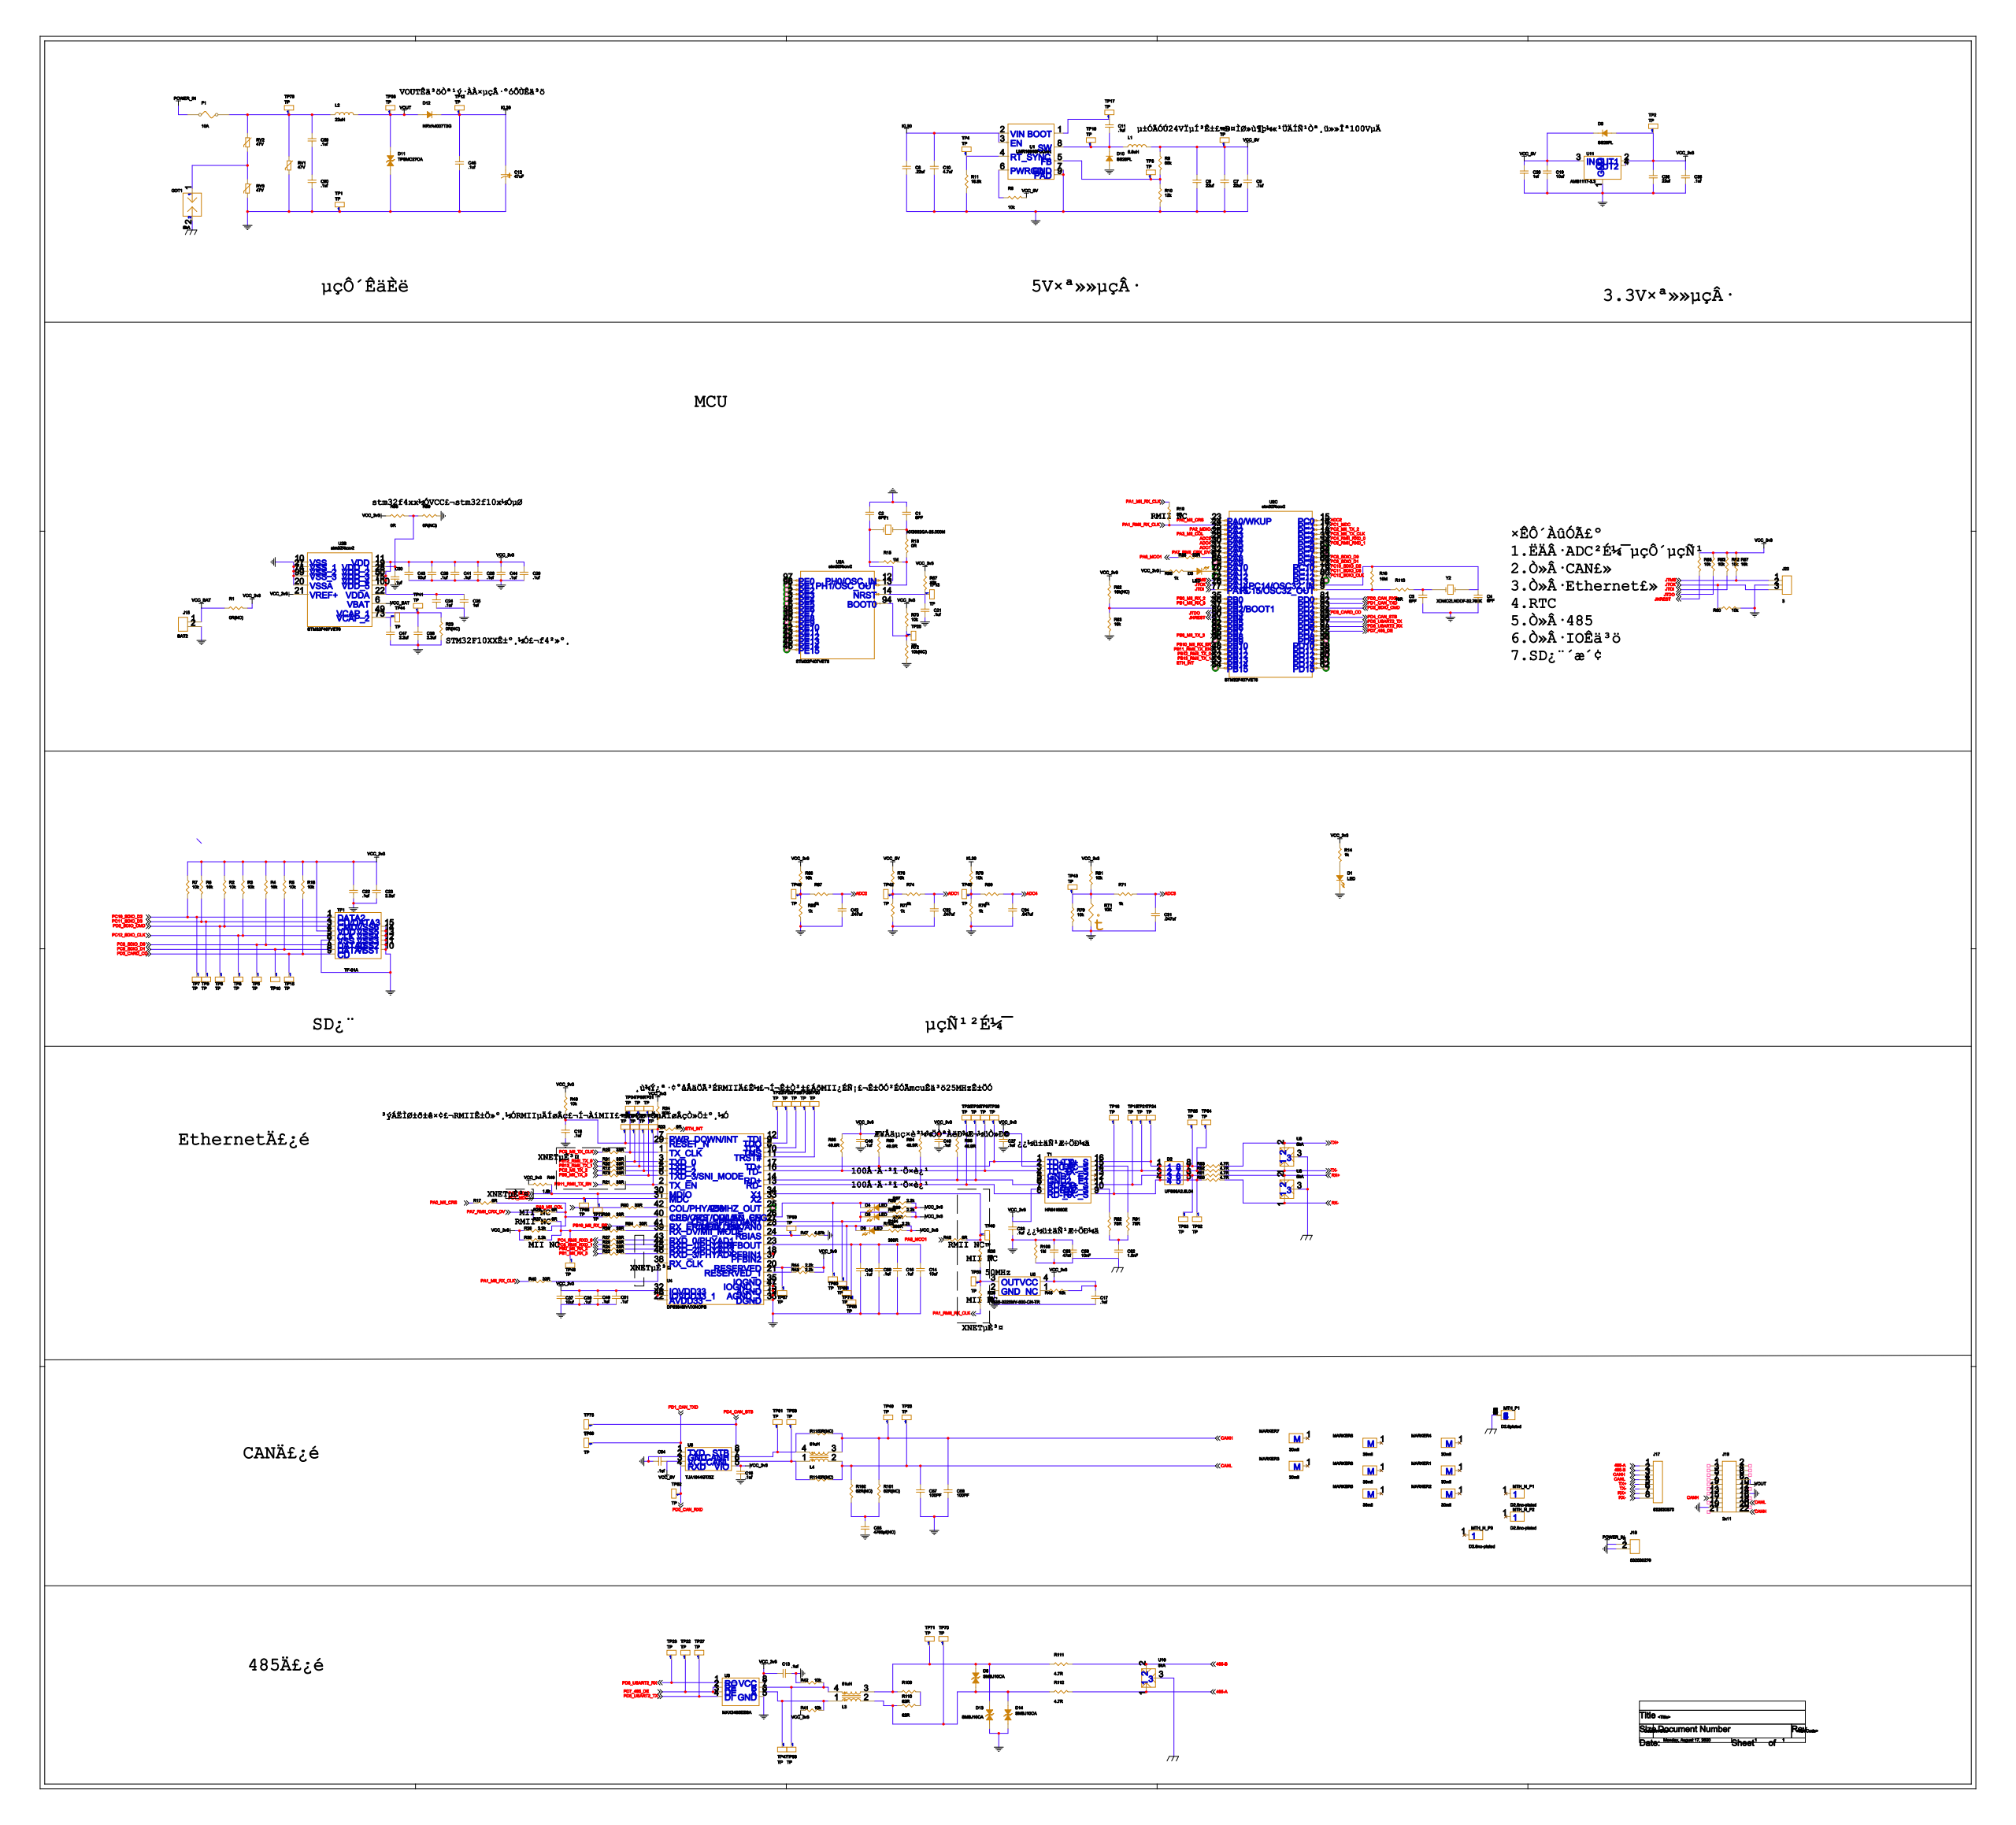Circuit board | Cadence Allegro | 279 parts | 142 nets
Bill of materials:
SYM_NAME,COMP_DEVICE_TYPE,COMP_VALUE,COMP_TOL,COMP_CLASS,REFDES
C0402,CAP_NP_C0402_8PF,8PF,,IC,C1
C0402,CAP_NP_C0402_8PF,8PF,,IC,C2
C0402,CAP_NP_C0402_6PF,6PF,,IC,C3
C0402,CAP_NP_C0402_6PF,6PF,,IC,C4
C1210,CAP_NP_C1210_22UF,22uf,,IC,C6
C1210,CAP_NP_C1210_22UF,22uf,,IC,C7
C0805,CAP_NP_C0805_.22UF,.22uf,,IC,C8
C0402,CAP_NP_C0402_.1UF,.1uf,,IC,C9
C1210,CAP_NP_C1210_4.7UF,4.7uf,,IC,C10
C0402,CAP_NP_C0402_.1UF,.1uf,,IC,C11
CAPAE630X770N,CAP_POL_CAPAE630X770N_47UF,47uF,,IC,C12
C0402,CAP_NP_C0402_.1UF,.1uf,,IC,C13
C1210,CAP_NP_C1210_10UF,10uf,,IC,C14
C0402,CAP_NP_C0402_.1UF,.1uf,,IC,C15
C0402,CAP_NP_C0402_.1UF,.1uf,,IC,C16
C0402,CAP_NP_C0402_.1UF,.1uf,,IC,C17
C0402,CAP_NP_C0402_.1UF,.1uf,,IC,C18
C1210,CAP_NP_C1210_10UF,10uf,,IC,C19
C0603,CAP_NP_C0603_1UF,1uf,,IC,C20
C0402,CAP_NP_C0402_.1UF,.1uf,,IC,C21
C0402,CAP_NP_C0402_.1UF,.1uf,,IC,C22
C0603,CAP_NP_C0603_2.2UF,2.2uf,,IC,C23
C0402,CAP_NP_C0402_.1UF,.1uf,,IC,C24
C0603,CAP_NP_C0603_1UF,1uf,,IC,C25
C0402,CAP_NP_C0402_.1UF,.1uf,,IC,C26
C0402,CAP_NP_C0402_.1UF,.1uf,,IC,C27
C0402,CAP_NP_C0402_.1UF,.1uf,,IC,C28
C0402,CAP_NP_C0402_.1UF,.1uf,,IC,C29
C0402,CAP_NP_C0402_.1UF,.1uf,,IC,C30
C0402,CAP_NP_C0402_.047UF,.047uf,,IC,C31
C0402,CAP_NP_C0402_.047UF,.047uf,,IC,C32
C0402,CAP_NP_C0402_.1UF,.1uf,,IC,C33
C0402,CAP_NP_C0402_.047UF,.047uf,,IC,C34
C0402,CAP_NP_C0402_.1UF,.1uf,,IC,C35
C1210,CAP_NP_C1210_22UF,22uf,,IC,C36
C1210,CAP_NP_C1210_10UF,10uf,,IC,C37
C0603,CAP_NP_C0603_2.2UF,2.2uf,,IC,C38
C0402,CAP_NP_C0402_.1UF,.1uf,,IC,C39
C0402,CAP_NP_C0402_.1UF,.1uf,,IC,C40
C0402,CAP_NP_C0402_.1UF,.1uf,,IC,C41
C0402,CAP_NP_C0402_.047UF,.047uf,,IC,C42
C1210,CAP_NP_C1210_10UF,10uf,,IC,C43
C0402,CAP_NP_C0402_.1UF,.1uf,,IC,C44
C0402,CAP_NP_C0402_.1UF,.1uf,,IC,C45
C0402,CAP_NP_C0402_.1UF,.1uf,,IC,C46
C0603,CAP_NP_C0603_2.2UF,2.2uf,,IC,C47
C0805,CAP_NP_C0805_.1UF,.1uf,,IC,C48
C0402,CAP_NP_C0402_.1UF,.1uf,,IC,C49
C0402,CAP_NP_C0402_.1UF,.1uf,,IC,C50
C0402,CAP_NP_C0402_.1UF,.1uf,,IC,C51
C1206,CAP_NP_C1206_1.5NF,1.5nF,,IC,C52
C1210,CAP_NP_C1210_47NF,47nf,,IC,C53
C0402,CAP_NP_C0402_.1UF,.1uf,,IC,C54
C0603,CAP_NP_C0603_4700PF(NC),4700pf(NC),,IC,C55
C1206,CAP_NP_C1206_10NF,10nF,,IC,C56
C0603,CAP_NP_C0603_100PF,100PF,,IC,C57
C0603,CAP_NP_C0603_100PF,100PF,,IC,C58
C0805,CAP_NP_C0805_.1UF,.1uf,,IC,C59
C0805,CAP_NP_C0805_.1UF,.1uf,,IC,C60
LED0603,LED_LED0603_LED,LED,,IC,D1
SOIC127P600X175-8N,ETH_TVS_SOIC127P600X175-8N_UFS0,UFS08A2.8L04,,IC,D2
LED0603,LED_LED0603_LED,LED,,IC,D3
LED0603,LED_LED0603_LED,LED,,IC,D4
LED0603,LED_LED0603_LED,LED,,IC,D5
LED0603,LED_LED0603_LED,LED,,IC,D6
SMB,TVS_BI_SMB_SMBJ10CA,SMBJ10CA,,IC,D8
SMA,DIODE_SMA_SS26FL,SS26FL,,IC,D9
SMA,DIODE_SMA_SS26FL,SS26FL,,IC,D10
SMC,TVS_BI_SMC_TPSMC27CA,TPSMC27CA,,IC,D11
SMA,DIODE_SMA_NRVA4007T3G,NRVA4007T3G,,IC,D12
SMB,TVS_BI_SMB_SMBJ10CA,SMBJ10CA,,IC,D13
SMB,TVS_BI_SMB_SMBJ10CA,SMBJ10CA,,IC,D14
FUSE10A,FUSE_FUSE10A_10A,10A,,IC,F1
GDT5KA2P,GDT_GDT5KA2P_5KA,5kA,,IC,GDT1
CR1220,CON2_CR1220_BAT2,BAT2,,IC,J15
532530870,CON8_532530870_532530870,532530870,,IC,J17
532530270,CON2_532530270_532530270,532530270,,IC,J18
CON2X11X200,CON2X11_CON2X11X200_2X11,2x11,,IC,J19
CON3X254,CON3_CON3X254_3,3,,IC,J20
SPM5030,INDUCTOR_SPM5030_6.8UH,6.8uH,,IC,L1
SPM6530,INDUCTOR_SPM6530_22UH,22uH,,IC,L2
CM320X450X150-4N,CHOKE CM14_CM320X450X150-4N_51U,51uH,,IC,L3
CM320X450X150-4N,CHOKE CM14_CM320X450X150-4N_51U,51uH,,IC,L4
FIDMS0,MARKER_FIDMS0_30MIL,30mil,,IC,MARKER1
FIDMS0,MARKER_FIDMS0_30MIL,30mil,,IC,MARKER2
FIDMS0,MARKER_FIDMS0_30MIL,30mil,,IC,MARKER3
FIDMS0,MARKER_FIDMS0_30MIL,30mil,,IC,MARKER4
FIDMS0,MARKER_FIDMS0_30MIL,30mil,,IC,MARKER5
FIDMS0,MARKER_FIDMS0_30MIL,30mil,,IC,MARKER6
FIDMS0,MARKER_FIDMS0_30MIL,30mil,,IC,MARKER7
FIDMS0,MARKER_FIDMS0_30MIL,30mil,,IC,MARKER8
MTGNP600H280Z380P,MTH_NO_PLATED_MTGNP600H280Z380P,D2.8no-plated,,IC,MTH_N_P1
MTGNP600H280Z380P,MTH_NO_PLATED_MTGNP600H280Z380P,D2.8no-plated,,IC,MTH_N_P2
MTGNP600H280Z380P,MTH_NO_PLATED_MTGNP600H280Z380P,D2.8no-plated,,IC,MTH_N_P3
MTGP6000H280V6P,MTH_PLATED_MTGP6000H280V6P_D2.8,D2.8plated,,IC,MTH_P1
R0402,R0402_R0402_0R(NC),0R(NC),,IC,R1
R0402,R0402_R0402_10K,10k,,DISCRETE,R2
R0402,R0402_R0402_10K,10k,,DISCRETE,R3
R0402,R0402_R0402_10K,10k,,DISCRETE,R4
R0402,R0402_R0402_10K,10k,,DISCRETE,R5
R0402,R0402_R0402_10K,10k,,DISCRETE,R6
R0402,R0402_R0402_10K,10k,,DISCRETE,R7
R0402,R0402_R0402_10K,10k,,DISCRETE,R8
R0402,R0402_R0402_68K,68k,,IC,R9
R0402,R0402_R0402_12K,12k,,IC,R10
R0402,R0402_R0402_16.9K,16.9k,,IC,R11
R0402,R0402_R0402_33R,33R,,DISCRETE,R12
R0402,R0402_R0402_0R,0R,,DISCRETE,R13
R0603,R0603_R0603_1K,1k,,IC,R14
R0402,R0402_R0402_1M,1M,,IC,R15
R0402,R0402_R0402_10M,10M,,IC,R16
R0402,R0402_R0402_0R,0R,,DISCRETE,R17
R0402,R0402_R0402_10K,10k,,DISCRETE,R18
R0402,R0402_R0402_0R,0R,,DISCRETE,R19
R0402,R0402_R0402_33R,33R,,DISCRETE,R20
R0402,R0402_R0402_33R,33R,,DISCRETE,R21
R0402,R0402_R0402_33R,33R,,DISCRETE,R22
R0402,R0402_R0402_0R(NC),0R(NC),,IC,R23
R0402,R0402_R0402_33R,33R,,DISCRETE,R24
R0402,R0402_R0402_33R,33R,,DISCRETE,R25
R0402,R0402_R0402_2.2K,2.2k,,IC,R26
R0402,R0402_R0402_33R,33R,,DISCRETE,R27
R0402,R0402_R0402_0R,0R,,DISCRETE,R28
R0402,R0402_R0402_0R,0R,,DISCRETE,R29
R0402,R0402_R0402_33R,33R,,DISCRETE,R30
R0402,R0402_R0402_33R,33R,,DISCRETE,R31
R0402,R0402_R0402_33R,33R,,DISCRETE,R32
R0402,R0402_R0402_0R,0R,,DISCRETE,R33
R0402,R0402_R0402_10K,10k,,DISCRETE,R34
R0402,R0402_R0402_33R,33R,,DISCRETE,R35
R0402,R0402_R0402_0R,0R,,DISCRETE,R36
R0402,R0402_R0402_0R,0R,,DISCRETE,R37
R0402,R0402_R0402_33R,33R,,DISCRETE,R38
R0402,R0402_R0402_2.2K,2.2k,,IC,R39
R0402,R0402_R0402_33R,33R,,DISCRETE,R40
R0402,R0402_R0402_10K,10k,,DISCRETE,R41
R0402,R0402_R0402_10K,10k,,DISCRETE,R42
R0402,R0402_R0402_2.2K,2.2k,,IC,R43
R0402,R0402_R0402_2.2K,2.2k,,IC,R44
R0402,R0402_R0402_10K,10k,,DISCRETE,R45
R0402,R0402_R0402_0R,0R,,DISCRETE,R46
R0402,R0402_R0402_4.87K,4.87k,,IC,R47
R0402,R0402_R0402_10K,10k,,DISCRETE,R48
R0402,R0402_R0402_1.5K,1.5k,,DISCRETE,R49
R1206,R1206_R1206_4.7R,4.7R,,IC,R50
R1206,R1206_R1206_4.7R,4.7R,,IC,R51
R1206,R1206_R1206_4.7R,4.7R,,IC,R52
R1206,R1206_R1206_4.7R,4.7R,,IC,R53
R0402,R0402_R0402_10K,10k,,DISCRETE,R57
R0402,R0402_R0402_10K,10k,,DISCRETE,R60
R0402,R0402_R0402_10K,10k,,DISCRETE,R62
R0402,R0402_R0402_10K,10k,,DISCRETE,R63
R0402,R0402_R0402_10K,10k,,DISCRETE,R65
R0402,R0402_R0402_10K,10k,,DISCRETE,R67
R0402,R0402_R0402_0R,0R,,DISCRETE,R68
R0402,R0402_R0402_0R(NC),0R(NC),,IC,R69
R0402,R0402_R0402_10K,10k,,DISCRETE,R70
R0402,R0402_R0402_1K,1k,,IC,R71
R0402,R0402_R0402_10K(NC),10k(NC),,IC,R72
R0402,R0402_R0402_33R,33R,,DISCRETE,R73
R0402,R0402_R0402_1K,1k,,IC,R74
R0402,R0402_R0402_1K,1k,,IC,R75
R0402,R0402_R0402_10K,10k,,DISCRETE,R76
R0402,R0402_R0402_1K,1k,,IC,R77
R0402,R0402_R0402_10K,10k,,DISCRETE,R78
R0402,R0402_R0402_10K,10k,,DISCRETE,R79
R0402,R0402_R0402_1K,1k,,IC,R80
R0402,R0402_R0402_10K,10k,,DISCRETE,R81
R0402,R0402_R0402_10K(NC),10k(NC),,IC,R82
R0402,R0402_R0402_10K,10k,,DISCRETE,R83
R0603,R0603_R0603_49.9R,49.9R,,IC,R84
R0603,R0603_R0603_49.9R,49.9R,,IC,R85
R0603,R0603_R0603_49.9R,49.9R,,IC,R86
R0402,R0402_R0402_1K,1k,,IC,R87
R0402,R0402_R0402_10K,10k,,DISCRETE,R88
R0603,R0603_R0603_49.9R,49.9R,,IC,R89
R0402,R0402_R0402_33R,33R,,DISCRETE,R90
R0603,R0603_R0603_75R,75R,,IC,R91
R0603,R0603_R0603_75R,75R,,IC,R92
R0402,R0402_R0402_1K,1k,,IC,R93
R0402,R0402_R0402_33R,33R,,DISCRETE,R94
R0603,R0603_R0603_1K,1k,,IC,R95
R0402,R0402_R0402_2.2K,2.2k,,IC,R96
R0805,R0805_R0805_390R,390R,,IC,R97
R0402,R0402_R0402_2.2K,2.2k,,IC,R98
R0805,R0805_R0805_390R,390R,,IC,R99
R1206,R1206_R1206_62R(NC),62R(NC),,IC,R101
R1206,R1206_R1206_62R(NC),62R(NC),,IC,R102
R0402,R0402_R0402_2.2K,2.2k,,IC,R103
R0805,R0805_R0805_390R,390R,,IC,R104
R1206,R1206_R1206_1M,1M,,IC,R106
R1206,R1206_R1206_62R,62R,,IC,R109
R1206,R1206_R1206_62R,62R,,IC,R110
R1206,R1206_R1206_4.7R,4.7R,,IC,R111
R1206,R1206_R1206_4.7R,4.7R,,IC,R112
R0402,R0402_R0402_10R,10R,,IC,R113
R0402,R0402_R0402_0R(NC),0R(NC),,IC,R114
R0402,R0402_R0402_0R(NC),0R(NC),,IC,R115
R0603,THERMISTOR_R0603_10K,10K,,IC,RT1
R2220,VARISTOR SYM_R2220_47V,47V,,IC,RV1
R2220,VARISTOR SYM_R2220_47V,47V,,IC,RV2
R2220,VARISTOR SYM_R2220_47V,47V,,IC,RV3
H1102,H1102_H1102_HR641680E,HR641680E,,IC,T1
TF-01A,TF_TF-01A_TF-01A,TF-01A,,IC,TF1
TPAD_30MIL,TP_TPAD_30MIL_TP,TP,,DISCRETE,TP1
TPAD_30MIL,TP_TPAD_30MIL_TP,TP,,DISCRETE,TP2
TPAD_30MIL,TP_TPAD_30MIL_TP,TP,,DISCRETE,TP3
TPAD_30MIL,TP_TPAD_30MIL_TP,TP,,DISCRETE,TP4
TPAD_30MIL,TP_TPAD_30MIL_TP,TP,,DISCRETE,TP5
TPAD_30MIL,TP_TPAD_30MIL_TP,TP,,DISCRETE,TP6
TPAD_30MIL,TP_TPAD_30MIL_TP,TP,,DISCRETE,TP7
TPAD_30MIL,TP_TPAD_30MIL_TP,TP,,DISCRETE,TP8
TPAD_30MIL,TP_TPAD_30MIL_TP,TP,,DISCRETE,TP9
TPAD_30MIL,TP_TPAD_30MIL_TP,TP,,DISCRETE,TP10
TPAD_30MIL,TP_TPAD_30MIL_TP,TP,,DISCRETE,TP11
TPAD_30MIL,TP_TPAD_30MIL_TP,TP,,DISCRETE,TP12
TPAD_30MIL,TP_TPAD_30MIL_TP,TP,,DISCRETE,TP13
TPAD_30MIL,TP_TPAD_30MIL_TP,TP,,DISCRETE,TP14
TPAD_30MIL,TP_TPAD_30MIL_TP,TP,,DISCRETE,TP15
TPAD_30MIL,TP_TPAD_30MIL_TP,TP,,DISCRETE,TP16
TPAD_30MIL,TP_TPAD_30MIL_TP,TP,,DISCRETE,TP17
TPAD_30MIL,TP_TPAD_30MIL_TP,TP,,DISCRETE,TP18
TPAD_30MIL,TP_TPAD_30MIL_TP,TP,,DISCRETE,TP19
TPAD_30MIL,TP_TPAD_30MIL_TP,TP,,DISCRETE,TP20
TPAD_30MIL,TP_TPAD_30MIL_TP,TP,,DISCRETE,TP21
TPAD_30MIL,TP_TPAD_30MIL_TP,TP,,DISCRETE,TP22
TPAD_30MIL,TP_TPAD_30MIL_TP,TP,,DISCRETE,TP23
TPAD_30MIL,TP_TPAD_30MIL_TP,TP,,DISCRETE,TP24
TPAD_30MIL,TP_TPAD_30MIL_TP,TP,,DISCRETE,TP25
TPAD_30MIL,TP_TPAD_30MIL_TP,TP,,DISCRETE,TP26
TPAD_30MIL,TP_TPAD_30MIL_TP,TP,,DISCRETE,TP27
TPAD_30MIL,TP_TPAD_30MIL_TP,TP,,DISCRETE,TP28
TPAD_30MIL,TP_TPAD_30MIL_TP,TP,,DISCRETE,TP29
TPAD_30MIL,TP_TPAD_30MIL_TP,TP,,DISCRETE,TP30
TPAD_30MIL,TP_TPAD_30MIL_TP,TP,,DISCRETE,TP31
TPAD_30MIL,TP_TPAD_30MIL_TP,TP,,DISCRETE,TP32
TPAD_30MIL,TP_TPAD_30MIL_TP,TP,,DISCRETE,TP33
TPAD_30MIL,TP_TPAD_30MIL_TP,TP,,DISCRETE,TP34
TPAD_30MIL,TP_TPAD_30MIL_TP,TP,,DISCRETE,TP35
TPAD_30MIL,TP_TPAD_30MIL_TP,TP,,DISCRETE,TP36
TPAD_30MIL,TP_TPAD_30MIL_TP,TP,,DISCRETE,TP37
TPAD_30MIL,TP_TPAD_30MIL_TP,TP,,DISCRETE,TP38
TPAD_30MIL,TP_TPAD_30MIL_TP,TP,,DISCRETE,TP39
TPAD_30MIL,TP_TPAD_30MIL_TP,TP,,DISCRETE,TP40
TPAD_30MIL,TP_TPAD_30MIL_TP,TP,,DISCRETE,TP41
TPAD_30MIL,TP_TPAD_30MIL_TP,TP,,DISCRETE,TP42
TPAD_30MIL,TP_TPAD_30MIL_TP,TP,,DISCRETE,TP43
TPAD_30MIL,TP_TPAD_30MIL_TP,TP,,DISCRETE,TP44
TPAD_30MIL,TP_TPAD_30MIL_TP,TP,,DISCRETE,TP45
TPAD_30MIL,TP_TPAD_30MIL_TP,TP,,DISCRETE,TP46
TPAD_30MIL,TP_TPAD_30MIL_TP,TP,,DISCRETE,TP47
TPAD_30MIL,TP_TPAD_30MIL_TP,TP,,DISCRETE,TP48
TPAD_30MIL,TP_TPAD_30MIL_TP,TP,,DISCRETE,TP49
TPAD_30MIL,TP_TPAD_30MIL_TP,TP,,DISCRETE,TP50
TPAD_30MIL,TP_TPAD_30MIL_TP,TP,,DISCRETE,TP51
TPAD_30MIL,TP_TPAD_30MIL_TP,TP,,DISCRETE,TP52
TPAD_30MIL,TP_TPAD_30MIL_TP,TP,,DISCRETE,TP53
TPAD_30MIL,TP_TPAD_30MIL_TP,TP,,DISCRETE,TP55
TPAD_30MIL,TP_TPAD_30MIL_TP,TP,,DISCRETE,TP56
TPAD_30MIL,TP_TPAD_30MIL_TP,TP,,DISCRETE,TP57
TPAD_30MIL,TP_TPAD_30MIL_TP,TP,,DISCRETE,TP58
TPAD_30MIL,TP_TPAD_30MIL_TP,TP,,DISCRETE,TP59
TPAD_30MIL,TP_TPAD_30MIL_TP,TP,,DISCRETE,TP60
TPAD_30MIL,TP_TPAD_30MIL_TP,TP,,DISCRETE,TP61
TPAD_30MIL,TP_TPAD_30MIL_TP,TP,,DISCRETE,TP62
TPAD_30MIL,TP_TPAD_30MIL_TP,TP,,DISCRETE,TP63
TPAD_30MIL,TP_TPAD_30MIL_TP,TP,,DISCRETE,TP64
TPAD_30MIL,TP_TPAD_30MIL_TP,TP,,DISCRETE,TP65
TPAD_30MIL,TP_TPAD_30MIL_TP,TP,,DISCRETE,TP66
TPAD_30MIL,TP_TPAD_30MIL_TP,TP,,DISCRETE,TP67
TPAD_30MIL,TP_TPAD_30MIL_TP,TP,,DISCRETE,TP68
TPAD_30MIL,TP_TPAD_30MIL_TP,TP,,DISCRETE,TP69
TPAD_30MIL,TP_TPAD_30MIL_TP,TP,,DISCRETE,TP70
TPAD_30MIL,TP_TPAD_30MIL_TP,TP,,DISCRETE,TP71
TPAD_30MIL,TP_TPAD_30MIL_TP,TP,,DISCRETE,TP72
TPAD_30MIL,TP_TPAD_30MIL_TP,TP,,DISCRETE,TP73
TPAD_30MIL,TP_TPAD_30MIL_TP,TP,,DISCRETE,TP74
TPAD_30MIL,TP_TPAD_30MIL_TP,TP,,DISCRETE,TP76
DDA0008E_N,LMR16010PDDAR_DDA0008E_N_LMR160,LMR16010PDDAR,,IC,U1
LQFP100-14X14MM,STM32F4XXV2_LQFP100-14X14MM_STM,STM32F407VET6,,IC,U2
SOIC127P600X175-8N,SP485EEN-L/TR_SOIC127P600X175-8,MAX3485EESA,,IC,U3
VBH48A_N,DP83848I_PT_48_VBH48A_N_DP83848,DP83848IVVX/NOPB,,IC,U4
OSCSC210P250X320X110-4N,Y_OSCSC210P250X320X110-4N_ECS-3,ECS-3225MV-500-CN-TR,,IC,U5
SOIC127P600X175-8N,TJA1044GT/3Z_SOIC127P600X175-8N,TJA1044GT/3Z,,IC,U6
GDT3P,GDTCM_GDT3P_5KA,5kA,,IC,U8
GDT3P,GDTCM_GDT3P_5KA,5kA,,IC,U9
GDT3P,GDTCM_GDT3P_5KA,5kA,,IC,U10
SOT223,AMS1117-3.3_SOT223_AMS1117-3.3,AMS1117-3.3,,IC,U11
XTAL500X320X150N,XTAL_XTAL500X320X150N_NX5032GA-,NX5032GA-25.000M,,IC,Y1
XTAL320X150X90N,XTAL_XTAL320X150X90N_XDMCZLNDDF,XDMCZLNDDF-32.768K,,IC,Y2
Netlist (net: part-pin ...):
KL30: C8-1 C10-1 C12-1 C48-1 D12-1 R76-1 TP12-1 U1-2 U1-3
GND: C1-1 C2-1 C3-2 C4-2 C6-2 C7-2 C8-2 C9-2 C10-2 C12-2 C13-2 C14-2 C15-2 C16-2 C17-2 C18-2 C19-2 C20-2 C21-2 C22-2 C23-2 C24-2 C25-2 C26-2 C27-2 C28-2 C29-2 C30-2 C31-2 C32-2 C33-2 C34-2 C35-2 C36-2 C37-2 C38-2 C39-2 C40-2 C41-2 C42-2 C43-2 C44-2 C45-2 C46-2 C47-2 C48-2 C49-2 C50-2 C51-2 C53-1 C54-1 C55-2 C56-1 C57-2 C58-2 C60-2 D1-1 D10-2 D11-1 D13-1 D14-1 J15-2 J18-2 J19-14 J19-19 J20-2 R10-2 R11-2 R23-2 R42-1 R47-2 R60-2 R69-2 R72-2 R75-1 R77-1 R79-2 R83-2 R93-1 R106-1 RT1-2 RV1-2 RV3-2 TF1-6 TF1-10 TF1-11 TF1-12 TF1-13 TF1-14 TF1-15 TP1-1 U1-7 U1-9 U2-10 U2-20 U2-27 U2-74 U2-99 U3-5 U4-15 U4-19 U4-35 U4-36 U4-47 U5-2 U6-2 U11-1
N00275: C59-1 F1-2 L2-1 RV1-1 RV2-1 TP76-1
N293431: C59-2 C60-1
N18571: C55-1 R101-2 R102-2
485-A: J17-1 R112-2 U10-1
485-B: J17-2 R111-2 U10-2
CANH: C58-1 J17-3 J19-15 J19-22 L4-3 R101-1 R115-2 TP40-1
CANL: C57-1 J17-4 J19-18 L4-2 R102-1 R114-2 TP33-1
TX+: J17-5 R53-2 U9-2
TX-: J17-6 R52-2 U9-1
RX+: J17-7 R51-2 U8-2
RX-: J17-8 R50-2 U8-1
POWER_IN: F1-1 J18-1
JTMS: J20-1 R57-2 U2-72
JTCK: J20-3 R60-1 U2-76
VOUT: D11-2 D12-2 J19-8 J19-10 L2-2 TP38-1
VCC_BAT: J15-1 R1-1 U2-6
GND_EARTH: C52-2 C53-2 C56-2 GDT1-2 MTH_P1-1 MTH_P1-2 MTH_P1-3 MTH_P1-4 MTH_P1-5 MTH_P1-6 MTH_P1-7 R106-2 U8-3 U9-3 U10-3
N161980: D6-2 R104-1
VCC_3V3: C13-1 C16-1 C17-1 C22-1 C23-1 C24-1 C25-1 C26-1 C27-1 C28-1 C29-1 C33-1 C35-1 C36-1 C37-1 C39-1 C40-1 C41-1 C43-1 C44-1 C46-1 C49-1 C51-1 D9-2 R1-2 R2-1 R3-1 R4-1 R5-1 R6-1 R7-1 R14-1 R18-1 R26-1 R34-1 R39-1 R41-1 R43-2 R44-2 R45-2 R48-1 R49-1 R57-1 R62-1 R63-1 R65-1 R67-1 R68-1 R70-1 R81-1 R82-1 R84-2 R85-2 R86-2 R88-1 R89-2 R95-1 R96-2 R97-2 R98-2 R99-2 R103-2 R104-2 T1-2 T1-7 TF1-4 TP2-1 U2-11 U2-21 U2-22 U2-28 U2-50 U2-75 U2-100 U3-8 U4-22 U4-32 U4-48 U5-4 U6-5 U11-2 U11-4
N168060: D4-2 R97-1
N171500: D5-2 R99-1
N44491: R16-1 R113-1 U2-9
N43458: C3-1 R113-2 Y2-1
N43454: C4-1 R16-2 U2-8 Y2-2
N45177: C2-2 R15-1 U2-12 Y1-1
N45173: C1-2 R13-1 Y1-2
N187359: R90-2 U4-42
N15161: R30-2 U4-40
N16786: D4-1 R96-1 TP60-1 U4-26
N16753: D6-1 R103-1 TP74-1 U4-28
N17134: D5-1 R98-1 TP68-1 U4-27
PC1_MDC: TP66-1 U2-16 U4-31
PA2_MDIO: R49-2 TP72-1 U2-25 U4-30
N10675: C14-1 C15-1 C45-1 C50-1 TP55-1 U4-18 U4-23 U4-37
N189117: R33-1 R34-2 U4-7
N214499: R47-1 TP59-1 U4-24
N13375: R85-1 T1-6 TP36-1 U4-14
N13387: R84-1 T1-8 TP35-1 U4-13
N143600: R44-1 TP57-1 U4-20
N141158: R43-1 U4-21
N35550: C18-1 R48-2 TP67-1 U4-29
N15257: R27-2 U4-43
N15289: R25-2 U4-44
N187114: R24-2 U4-45
N187118: R22-2 U4-46
N187418: R40-2 U4-38
N15225: R38-2 U4-39
N187385: R94-2 U4-41
N205416: TP26-1 U4-8
N12660: R89-1 T1-1 TP39-1 U4-17
N12667: R86-1 T1-3 TP37-1 U4-16
N205402: TP32-1 U4-12
N205409: TP25-1 U4-9
N205423: TP28-1 U4-10
N205430: TP30-1 U4-11
N14786: R31-2 TP51-1 U4-3
N14816: R32-2 TP50-1 U4-4
N187307: R12-2 TP11-1 U4-5
N187303: R73-2 TP31-1 U4-6
N187333: R20-2 TP34-1 U4-1
N14912: R21-2 TP29-1 U4-2
N21007: R36-2 R46-2 TP49-1 U4-34
PD4_CAN_STB: TP73-1 U2-85 U6-8
N50670: D8-2 D13-2 L3-3 R109-1 R111-1 TP71-1
N50740: D8-1 D14-2 L3-2 R110-1 R112-1 TP70-1
PD1_CAN_TXD: TP69-1 U2-82 U6-1
N65708: D2-1 D2-8 R53-1 T1-16 TP24-1 TP65-1
N65715: D2-2 D2-7 R52-1 T1-14 TP21-1 TP64-1
N65719: D2-3 D2-6 R51-1 T1-11 TP18-1 TP63-1
N65763: D2-4 D2-5 R50-1 T1-9 TP16-1 TP62-1
N23776: L4-4 R115-1 TP61-1 U6-7
N23788: L4-1 R114-1 TP58-1 U6-6
N58601: L3-4 R42-2 TP56-1 U3-7
N33271: R28-2 R36-1 TP53-1 U5-3
PD0_CAN_RXD: TP52-1 U2-81 U6-4
N15077: R37-2 R38-1 R39-2 TP48-1
N58608: L3-1 R41-2 TP47-1 U3-6
N33320: R87-2 R88-2 R93-2 TP46-1
N34330: R75-2 R76-2 R80-2 TP45-1
N24615: C47-1 TP44-1 U2-73
N180678: R71-2 R79-1 R81-2 RT1-1 TP43-1
N33942: R74-2 R77-2 R78-2 TP42-1
N06616: C38-1 R23-1 TP41-1 U2-49
PD5_USART2_TX: TP27-1 U2-86 U3-4
PD6_USART2_RX: TP23-1 U2-87 U3-1
PD7_485_DE: TP22-1 U2-88 U3-2 U3-3
N28916: R70-2 R72-1 TP20-1 U2-94
N03413: C11-2 D10-1 L1-1 TP19-1 U1-8
N03401: C11-1 TP17-1 U1-1
PD3_CARD_CD: R18-2 TF1-9 TP15-1 U2-84
VCC_5V: C6-1 C7-1 C9-1 C19-1 C20-1 C54-2 D9-1 L1-2 R8-2 R9-1 R78-1 TP14-1 U6-3 U11-3
N06994: C21-1 R67-2 TP13-1 U2-14
PC9_SDIO_D1: R5-2 TF1-8 TP10-1 U2-66
PC11_SDIO_D3: R6-2 TF1-2 TP9-1 U2-79
PC12_SDIO_CLK: R3-2 TF1-5 TP8-1 U2-80
PC10_SDIO_D2: R7-2 TF1-1 TP7-1 U2-78
PD2_SDIO_CMD: R2-2 TF1-3 TP6-1 U2-83
PC8_SDIO_D0: R4-2 TF1-7 TP5-1 U2-65
N03576: R11-1 TP4-1 U1-4
N03507: R9-2 R10-1 TP3-1 U1-5
N02752: GDT1-1 RV2-2 RV3-1
N58846: R109-2 R110-2
N17429: R92-1 T1-10
N18419: C52-1 R91-2 R92-2
N17422: R91-1 T1-15
N2364511: D3-2 R95-2
N2359181: D1-2 R14-2
PB10_MII_RX_ER: R94-1 U2-47
PA3_MII_COL: R90-1 U2-26
PB8_MII_TX_3: R73-1 U2-95
PA1_MII_RX_CLK: R19-2 R40-1
PA8_MCO1: R35-1 R46-1
N187727: R35-2 U2-67
PB13_RMII_TX_1: R32-1 U2-52
PB12_RMII_TX_0: R31-1 U2-51
N15089: R17-2 R26-2 R29-2 R30-1
PC4_RMII_RXD_0: R27-1 U2-33
PC5_RMII_RXD_1: R25-1 U2-34
PB0_MII_RX_2: R24-1 U2-35
PB1_MII_RX_3: R22-1 U2-36
PB11_RMII_TX_EN: R21-1 U2-48
PC3_MII_TX_CLK: R20-1 U2-18
PC2_MII_TX_2: R12-1 U2-17
N29074: R82-2 R83-1 U2-37
JNREST: R65-2 U2-90
JTDO: R63-2 U2-89
JTDI: R62-2 U2-77
N961250: R45-1 U5-1
N04146: R8-1 U1-6
N45183: R13-2 R15-2 U2-13
ADC2: C42-1 R87-1 U2-15
ADC4: C34-1 R80-1 U2-30
ADC1: C32-1 R74-1 U2-31
ADC3: C31-1 R71-1 U2-29
N26484: C30-1 R68-2 R69-1 U2-19
PA7_RMII_CRX_DV: R29-1 R37-1 U2-32
ETH_INT: R33-2 U2-53
PA1_RMII_RX_CLK: R19-1 R28-1 U2-24
PA0_MII_CRS: R17-1 U2-23
N0228241: D3-1 U2-70